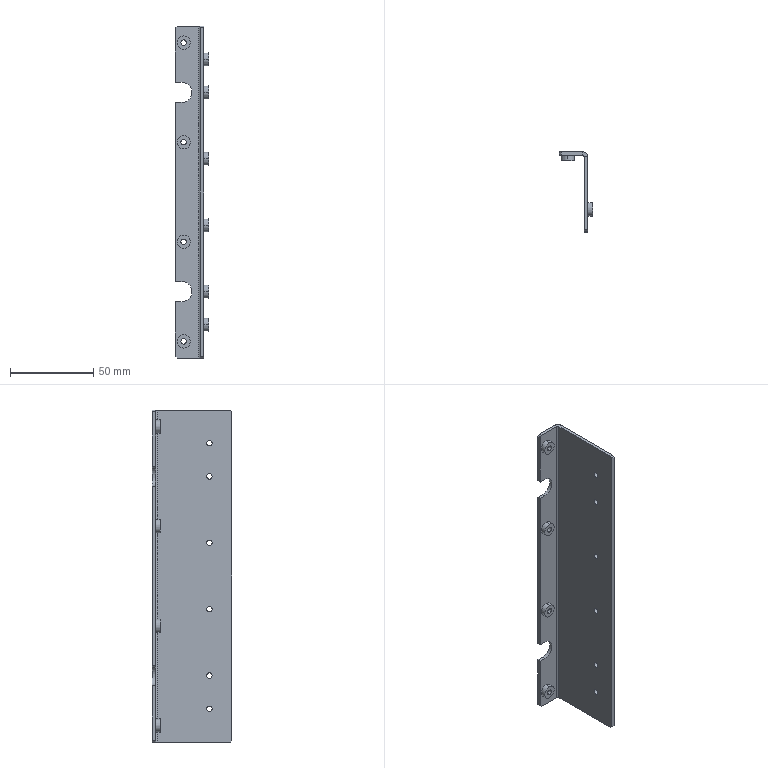Part | SolidWorks | features HoleWzd 2, ICE 2, Chamfer 1, Cut 1, EdgeFlange 1, FlatPattern 1, LPattern 1, SMBaseFlange 1, SheetMetal 1 | 1 solid | 76 faces | box 20 x 48 x 200 mm | volume 25515 mm3 | cylinder 44 | plane 32 | commonest cylinder face diameters 3.3 x20 8 x20 12 x2 2 x1 6 x1